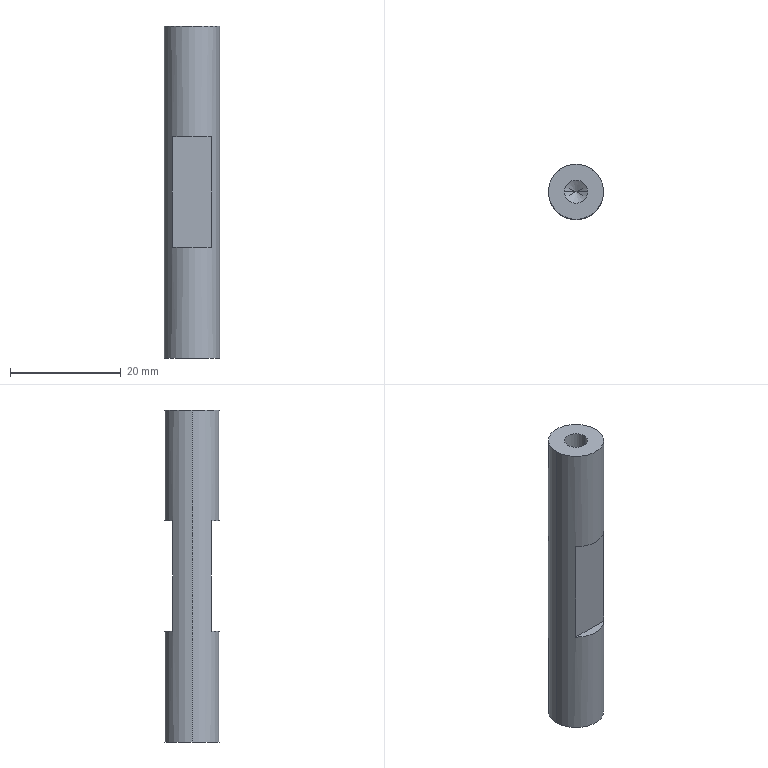Part | SolidWorks | features 3DProfileFeature 1, Extrusion 1, HoleWzd 1, ICE 1, MirrorPattern 1 | 1 solid | 18 faces | box 10 x 10 x 60 mm | volume 3990 mm3 | plane 8 | cylinder 6 | cone 4 | commonest cylinder face diameters 4.2 x4 10 x2
STEP:
#1=CARTESIAN_POINT('',(-87.9,55.,15.));
#2=VERTEX_POINT('',#1);
#3=CARTESIAN_POINT('',(-92.1,55.,15.));
#4=VERTEX_POINT('',#3);
#5=CARTESIAN_POINT('',(-90.,55.,15.));
#6=DIRECTION('',(0.,0.,-1.));
#7=DIRECTION('',(-1.,0.,0.));
#8=AXIS2_PLACEMENT_3D('',#5,#6,#7);
#9=CIRCLE('',#8,2.1);
#10=EDGE_CURVE('',#2,#4,#9,.T.);
#11=ORIENTED_EDGE('',*,*,#10,.F.);
#12=CARTESIAN_POINT('',(-87.9,55.,0.));
#13=VERTEX_POINT('',#12);
#14=CARTESIAN_POINT('',(-87.9,55.,0.));
#15=DIRECTION('',(0.,0.,-1.));
#16=VECTOR('',#15,1000.);
#17=LINE('',#14,#16);
#18=EDGE_CURVE('',#2,#13,#17,.T.);
#19=ORIENTED_EDGE('',*,*,#18,.T.);
#20=CARTESIAN_POINT('',(-92.1,55.,0.));
#21=VERTEX_POINT('',#20);
#22=CARTESIAN_POINT('',(-90.,55.,0.));
#23=DIRECTION('',(0.,0.,-1.));
#24=DIRECTION('',(-1.,0.,0.));
#25=AXIS2_PLACEMENT_3D('',#22,#23,#24);
#26=CIRCLE('',#25,2.1);
#27=EDGE_CURVE('',#13,#21,#26,.T.);
#28=ORIENTED_EDGE('',*,*,#27,.T.);
#29=CARTESIAN_POINT('',(-92.1,55.,0.));
#30=DIRECTION('',(0.,0.,-1.));
#31=VECTOR('',#30,1000.);
#32=LINE('',#29,#31);
#33=EDGE_CURVE('',#4,#21,#32,.T.);
#34=ORIENTED_EDGE('',*,*,#33,.F.);
#35=EDGE_LOOP('',(#11,#19,#28,#34));
#36=FACE_OUTER_BOUND('',#35,.T.);
#37=CARTESIAN_POINT('',(-90.,55.,0.));
#38=DIRECTION('',(0.,0.,-1.));
#39=DIRECTION('',(-1.,0.,0.));
#40=AXIS2_PLACEMENT_3D('',#37,#38,#39);
#41=CYLINDRICAL_SURFACE('',#40,2.1);
#42=ADVANCED_FACE('',(#36),#41,.F.);
#43=CARTESIAN_POINT('',(-90.,55.,16.262));
#44=VERTEX_POINT('',#43);
#45=CARTESIAN_POINT('',(-92.1,55.,15.));
#46=DIRECTION('',(-0.8572,0.,-0.515));
#47=VECTOR('',#46,1000.);
#48=LINE('',#45,#47);
#49=EDGE_CURVE('',#44,#4,#48,.T.);
#50=ORIENTED_EDGE('',*,*,#49,.F.);
#51=CARTESIAN_POINT('',(-87.9,55.,15.));
#52=DIRECTION('',(0.8572,0.,-0.515));
#53=VECTOR('',#52,1000.);
#54=LINE('',#51,#53);
#55=EDGE_CURVE('',#44,#2,#54,.T.);
#56=ORIENTED_EDGE('',*,*,#55,.T.);
#57=ORIENTED_EDGE('',*,*,#10,.T.);
#58=EDGE_LOOP('',(#50,#56,#57));
#59=FACE_OUTER_BOUND('',#58,.T.);
#60=CARTESIAN_POINT('',(-90.,55.,15.));
#61=DIRECTION('',(0.,0.,-1.));
#62=DIRECTION('',(-1.,0.,0.));
#63=AXIS2_PLACEMENT_3D('',#60,#61,#62);
#64=CONICAL_SURFACE('',#63,2.1,1.03);
#65=ADVANCED_FACE('',(#59),#64,.F.);
#66=CARTESIAN_POINT('',(-92.1,55.,45.));
#67=VERTEX_POINT('',#66);
#68=CARTESIAN_POINT('',(-87.9,55.,45.));
#69=VERTEX_POINT('',#68);
#70=CARTESIAN_POINT('',(-90.,55.,45.));
#71=DIRECTION('',(0.,0.,1.));
#72=DIRECTION('',(1.,0.,0.));
#73=AXIS2_PLACEMENT_3D('',#70,#71,#72);
#74=CIRCLE('',#73,2.1);
#75=EDGE_CURVE('',#67,#69,#74,.T.);
#76=ORIENTED_EDGE('',*,*,#75,.F.);
#77=CARTESIAN_POINT('',(-92.1,55.,60.));
#78=VERTEX_POINT('',#77);
#79=CARTESIAN_POINT('',(-92.1,55.,60.));
#80=DIRECTION('',(0.,0.,1.));
#81=VECTOR('',#80,1000.);
#82=LINE('',#79,#81);
#83=EDGE_CURVE('',#67,#78,#82,.T.);
#84=ORIENTED_EDGE('',*,*,#83,.T.);
#85=CARTESIAN_POINT('',(-87.9,55.,60.));
#86=VERTEX_POINT('',#85);
#87=CARTESIAN_POINT('',(-90.,55.,60.));
#88=DIRECTION('',(0.,0.,1.));
#89=DIRECTION('',(1.,0.,0.));
#90=AXIS2_PLACEMENT_3D('',#87,#88,#89);
#91=CIRCLE('',#90,2.1);
#92=EDGE_CURVE('',#78,#86,#91,.T.);
#93=ORIENTED_EDGE('',*,*,#92,.T.);
#94=CARTESIAN_POINT('',(-87.9,55.,60.));
#95=DIRECTION('',(0.,0.,1.));
#96=VECTOR('',#95,1000.);
#97=LINE('',#94,#96);
#98=EDGE_CURVE('',#69,#86,#97,.T.);
#99=ORIENTED_EDGE('',*,*,#98,.F.);
#100=EDGE_LOOP('',(#76,#84,#93,#99));
#101=FACE_OUTER_BOUND('',#100,.T.);
#102=CARTESIAN_POINT('',(-90.,55.,60.));
#103=DIRECTION('',(0.,0.,1.));
#104=DIRECTION('',(1.,0.,0.));
#105=AXIS2_PLACEMENT_3D('',#102,#103,#104);
#106=CYLINDRICAL_SURFACE('',#105,2.1);
#107=ADVANCED_FACE('',(#101),#106,.F.);
#108=CARTESIAN_POINT('',(-90.,55.,43.738));
#109=VERTEX_POINT('',#108);
#110=CARTESIAN_POINT('',(-87.9,55.,45.));
#111=DIRECTION('',(0.8572,0.,0.515));
#112=VECTOR('',#111,1000.);
#113=LINE('',#110,#112);
#114=EDGE_CURVE('',#109,#69,#113,.T.);
#115=ORIENTED_EDGE('',*,*,#114,.F.);
#116=CARTESIAN_POINT('',(-92.1,55.,45.));
#117=DIRECTION('',(-0.8572,0.,0.515));
#118=VECTOR('',#117,1000.);
#119=LINE('',#116,#118);
#120=EDGE_CURVE('',#109,#67,#119,.T.);
#121=ORIENTED_EDGE('',*,*,#120,.T.);
#122=ORIENTED_EDGE('',*,*,#75,.T.);
#123=EDGE_LOOP('',(#115,#121,#122));
#124=FACE_OUTER_BOUND('',#123,.T.);
#125=CARTESIAN_POINT('',(-90.,55.,45.));
#126=DIRECTION('',(0.,0.,1.));
#127=DIRECTION('',(1.,0.,0.));
#128=AXIS2_PLACEMENT_3D('',#125,#126,#127);
#129=CONICAL_SURFACE('',#128,2.1,1.03);
#130=ADVANCED_FACE('',(#124),#129,.F.);
#131=CARTESIAN_POINT('',(-86.429,58.5,20.));
#132=VERTEX_POINT('',#131);
#133=CARTESIAN_POINT('',(-86.429,58.5,40.));
#134=VERTEX_POINT('',#133);
#135=CARTESIAN_POINT('',(-86.429,58.5,60.));
#136=DIRECTION('',(0.,0.,1.));
#137=VECTOR('',#136,1000.);
#138=LINE('',#135,#137);
#139=EDGE_CURVE('',#132,#134,#138,.T.);
#140=ORIENTED_EDGE('',*,*,#139,.T.);
#141=CARTESIAN_POINT('',(-93.571,58.5,40.));
#142=VERTEX_POINT('',#141);
#143=CARTESIAN_POINT('',(-90.,55.,40.));
#144=DIRECTION('',(0.,0.,1.));
#145=DIRECTION('',(1.,0.,0.));
#146=AXIS2_PLACEMENT_3D('',#143,#144,#145);
#147=CIRCLE('',#146,5.);
#148=EDGE_CURVE('',#134,#142,#147,.T.);
#149=ORIENTED_EDGE('',*,*,#148,.T.);
#150=CARTESIAN_POINT('',(-93.571,58.5,20.));
#151=VERTEX_POINT('',#150);
#152=CARTESIAN_POINT('',(-93.571,58.5,60.));
#153=DIRECTION('',(0.,0.,-1.));
#154=VECTOR('',#153,1000.);
#155=LINE('',#152,#154);
#156=EDGE_CURVE('',#142,#151,#155,.T.);
#157=ORIENTED_EDGE('',*,*,#156,.T.);
#158=CARTESIAN_POINT('',(-90.,55.,20.));
#159=DIRECTION('',(0.,0.,-1.));
#160=DIRECTION('',(-1.,0.,0.));
#161=AXIS2_PLACEMENT_3D('',#158,#159,#160);
#162=CIRCLE('',#161,5.);
#163=EDGE_CURVE('',#151,#132,#162,.T.);
#164=ORIENTED_EDGE('',*,*,#163,.T.);
#165=EDGE_LOOP('',(#140,#149,#157,#164));
#166=FACE_BOUND('',#165,.T.);
#167=CARTESIAN_POINT('',(-85.,55.,60.));
#168=VERTEX_POINT('',#167);
#169=CARTESIAN_POINT('',(-95.,55.,60.));
#170=VERTEX_POINT('',#169);
#171=CARTESIAN_POINT('',(-90.,55.,60.));
#172=DIRECTION('',(0.,0.,1.));
#173=DIRECTION('',(1.,0.,0.));
#174=AXIS2_PLACEMENT_3D('',#171,#172,#173);
#175=CIRCLE('',#174,5.);
#176=EDGE_CURVE('',#168,#170,#175,.T.);
#177=ORIENTED_EDGE('',*,*,#176,.F.);
#178=CARTESIAN_POINT('',(-85.,55.,0.));
#179=VERTEX_POINT('',#178);
#180=CARTESIAN_POINT('',(-85.,55.,60.));
#181=DIRECTION('',(0.,0.,-1.));
#182=VECTOR('',#181,1000.);
#183=LINE('',#180,#182);
#184=EDGE_CURVE('',#168,#179,#183,.T.);
#185=ORIENTED_EDGE('',*,*,#184,.T.);
#186=CARTESIAN_POINT('',(-95.,55.,0.));
#187=VERTEX_POINT('',#186);
#188=CARTESIAN_POINT('',(-90.,55.,0.));
#189=DIRECTION('',(0.,0.,1.));
#190=DIRECTION('',(1.,0.,0.));
#191=AXIS2_PLACEMENT_3D('',#188,#189,#190);
#192=CIRCLE('',#191,5.);
#193=EDGE_CURVE('',#179,#187,#192,.T.);
#194=ORIENTED_EDGE('',*,*,#193,.T.);
#195=CARTESIAN_POINT('',(-95.,55.,60.));
#196=DIRECTION('',(0.,0.,-1.));
#197=VECTOR('',#196,1000.);
#198=LINE('',#195,#197);
#199=EDGE_CURVE('',#170,#187,#198,.T.);
#200=ORIENTED_EDGE('',*,*,#199,.F.);
#201=EDGE_LOOP('',(#177,#185,#194,#200));
#202=FACE_OUTER_BOUND('',#201,.T.);
#203=CARTESIAN_POINT('',(-90.,55.,60.));
#204=DIRECTION('',(0.,0.,-1.));
#205=DIRECTION('',(-1.,0.,0.));
#206=AXIS2_PLACEMENT_3D('',#203,#204,#205);
#207=CYLINDRICAL_SURFACE('',#206,5.);
#208=ADVANCED_FACE('',(#166,#202),#207,.T.);
#209=ORIENTED_EDGE('',*,*,#184,.F.);
#210=CARTESIAN_POINT('',(-90.,55.,60.));
#211=DIRECTION('',(0.,0.,1.));
#212=DIRECTION('',(1.,0.,0.));
#213=AXIS2_PLACEMENT_3D('',#210,#211,#212);
#214=CIRCLE('',#213,5.);
#215=EDGE_CURVE('',#170,#168,#214,.T.);
#216=ORIENTED_EDGE('',*,*,#215,.F.);
#217=ORIENTED_EDGE('',*,*,#199,.T.);
#218=CARTESIAN_POINT('',(-90.,55.,0.));
#219=DIRECTION('',(0.,0.,1.));
#220=DIRECTION('',(1.,0.,0.));
#221=AXIS2_PLACEMENT_3D('',#218,#219,#220);
#222=CIRCLE('',#221,5.);
#223=EDGE_CURVE('',#187,#179,#222,.T.);
#224=ORIENTED_EDGE('',*,*,#223,.T.);
#225=EDGE_LOOP('',(#209,#216,#217,#224));
#226=FACE_OUTER_BOUND('',#225,.T.);
#227=CARTESIAN_POINT('',(-93.571,51.5,20.));
#228=VERTEX_POINT('',#227);
#229=CARTESIAN_POINT('',(-86.429,51.5,20.));
#230=VERTEX_POINT('',#229);
#231=CARTESIAN_POINT('',(-90.,55.,20.));
#232=DIRECTION('',(0.,0.,1.));
#233=DIRECTION('',(1.,0.,0.));
#234=AXIS2_PLACEMENT_3D('',#231,#232,#233);
#235=CIRCLE('',#234,5.);
#236=EDGE_CURVE('',#228,#230,#235,.T.);
#237=ORIENTED_EDGE('',*,*,#236,.F.);
#238=CARTESIAN_POINT('',(-93.571,51.5,40.));
#239=VERTEX_POINT('',#238);
#240=CARTESIAN_POINT('',(-93.571,51.5,60.));
#241=DIRECTION('',(0.,0.,1.));
#242=VECTOR('',#241,1000.);
#243=LINE('',#240,#242);
#244=EDGE_CURVE('',#228,#239,#243,.T.);
#245=ORIENTED_EDGE('',*,*,#244,.T.);
#246=CARTESIAN_POINT('',(-86.429,51.5,40.));
#247=VERTEX_POINT('',#246);
#248=CARTESIAN_POINT('',(-90.,55.,40.));
#249=DIRECTION('',(0.,0.,-1.));
#250=DIRECTION('',(-1.,0.,0.));
#251=AXIS2_PLACEMENT_3D('',#248,#249,#250);
#252=CIRCLE('',#251,5.);
#253=EDGE_CURVE('',#247,#239,#252,.T.);
#254=ORIENTED_EDGE('',*,*,#253,.F.);
#255=CARTESIAN_POINT('',(-86.429,51.5,60.));
#256=DIRECTION('',(0.,0.,-1.));
#257=VECTOR('',#256,1000.);
#258=LINE('',#255,#257);
#259=EDGE_CURVE('',#247,#230,#258,.T.);
#260=ORIENTED_EDGE('',*,*,#259,.T.);
#261=EDGE_LOOP('',(#237,#245,#254,#260));
#262=FACE_BOUND('',#261,.T.);
#263=CARTESIAN_POINT('',(-90.,55.,60.));
#264=DIRECTION('',(0.,0.,-1.));
#265=DIRECTION('',(-1.,0.,0.));
#266=AXIS2_PLACEMENT_3D('',#263,#264,#265);
#267=CYLINDRICAL_SURFACE('',#266,5.);
#268=ADVANCED_FACE('',(#226,#262),#267,.T.);
#269=CARTESIAN_POINT('',(-90.,55.,60.));
#270=DIRECTION('',(0.,0.,1.));
#271=DIRECTION('',(1.,0.,0.));
#272=AXIS2_PLACEMENT_3D('',#269,#270,#271);
#273=CIRCLE('',#272,2.1);
#274=EDGE_CURVE('',#86,#78,#273,.T.);
#275=ORIENTED_EDGE('',*,*,#274,.F.);
#276=ORIENTED_EDGE('',*,*,#92,.F.);
#277=EDGE_LOOP('',(#275,#276));
#278=FACE_BOUND('',#277,.T.);
#279=ORIENTED_EDGE('',*,*,#215,.T.);
#280=ORIENTED_EDGE('',*,*,#176,.T.);
#281=EDGE_LOOP('',(#279,#280));
#282=FACE_OUTER_BOUND('',#281,.T.);
#283=CARTESIAN_POINT('',(-90.,55.,60.));
#284=DIRECTION('',(0.,0.,1.));
#285=DIRECTION('',(1.,0.,0.));
#286=AXIS2_PLACEMENT_3D('',#283,#284,#285);
#287=PLANE('',#286);
#288=ADVANCED_FACE('',(#278,#282),#287,.T.);
#289=CARTESIAN_POINT('',(-90.,55.,0.));
#290=DIRECTION('',(0.,0.,-1.));
#291=DIRECTION('',(-1.,0.,0.));
#292=AXIS2_PLACEMENT_3D('',#289,#290,#291);
#293=CIRCLE('',#292,2.1);
#294=EDGE_CURVE('',#21,#13,#293,.T.);
#295=ORIENTED_EDGE('',*,*,#294,.F.);
#296=ORIENTED_EDGE('',*,*,#27,.F.);
#297=EDGE_LOOP('',(#295,#296));
#298=FACE_BOUND('',#297,.T.);
#299=ORIENTED_EDGE('',*,*,#223,.F.);
#300=ORIENTED_EDGE('',*,*,#193,.F.);
#301=EDGE_LOOP('',(#299,#300));
#302=FACE_OUTER_BOUND('',#301,.T.);
#303=CARTESIAN_POINT('',(-90.,55.,0.));
#304=DIRECTION('',(0.,0.,1.));
#305=DIRECTION('',(1.,0.,0.));
#306=AXIS2_PLACEMENT_3D('',#303,#304,#305);
#307=PLANE('',#306);
#308=ADVANCED_FACE('',(#298,#302),#307,.F.);
#309=CARTESIAN_POINT('',(-100.,58.5,40.));
#310=DIRECTION('',(1.,0.,0.));
#311=VECTOR('',#310,1000.);
#312=LINE('',#309,#311);
#313=EDGE_CURVE('',#142,#134,#312,.T.);
#314=ORIENTED_EDGE('',*,*,#313,.F.);
#315=ORIENTED_EDGE('',*,*,#148,.F.);
#316=EDGE_LOOP('',(#314,#315));
#317=FACE_OUTER_BOUND('',#316,.T.);
#318=CARTESIAN_POINT('',(-100.,58.5,40.));
#319=DIRECTION('',(0.,0.,1.));
#320=DIRECTION('',(1.,0.,0.));
#321=AXIS2_PLACEMENT_3D('',#318,#319,#320);
#322=PLANE('',#321);
#323=ADVANCED_FACE('',(#317),#322,.F.);
#324=CARTESIAN_POINT('',(-100.,58.5,20.));
#325=DIRECTION('',(-1.,0.,0.));
#326=VECTOR('',#325,1000.);
#327=LINE('',#324,#326);
#328=EDGE_CURVE('',#132,#151,#327,.T.);
#329=ORIENTED_EDGE('',*,*,#328,.F.);
#330=ORIENTED_EDGE('',*,*,#163,.F.);
#331=EDGE_LOOP('',(#329,#330));
#332=FACE_OUTER_BOUND('',#331,.T.);
#333=CARTESIAN_POINT('',(-100.,58.5,20.));
#334=DIRECTION('',(0.,0.,-1.));
#335=DIRECTION('',(-1.,0.,0.));
#336=AXIS2_PLACEMENT_3D('',#333,#334,#335);
#337=PLANE('',#336);
#338=ADVANCED_FACE('',(#332),#337,.F.);
#339=ORIENTED_EDGE('',*,*,#313,.T.);
#340=ORIENTED_EDGE('',*,*,#139,.F.);
#341=ORIENTED_EDGE('',*,*,#328,.T.);
#342=ORIENTED_EDGE('',*,*,#156,.F.);
#343=EDGE_LOOP('',(#339,#340,#341,#342));
#344=FACE_OUTER_BOUND('',#343,.T.);
#345=CARTESIAN_POINT('',(0.,58.5,0.));
#346=DIRECTION('',(0.,-1.,0.));
#347=DIRECTION('',(0.,0.,-1.));
#348=AXIS2_PLACEMENT_3D('',#345,#346,#347);
#349=PLANE('',#348);
#350=ADVANCED_FACE('',(#344),#349,.F.);
#351=CARTESIAN_POINT('',(-100.,51.5,20.));
#352=DIRECTION('',(-1.,0.,0.));
#353=VECTOR('',#352,1000.);
#354=LINE('',#351,#353);
#355=EDGE_CURVE('',#230,#228,#354,.T.);
#356=ORIENTED_EDGE('',*,*,#355,.T.);
#357=ORIENTED_EDGE('',*,*,#236,.T.);
#358=EDGE_LOOP('',(#356,#357));
#359=FACE_OUTER_BOUND('',#358,.T.);
#360=CARTESIAN_POINT('',(-100.,51.5,20.));
#361=DIRECTION('',(0.,0.,1.));
#362=DIRECTION('',(1.,0.,0.));
#363=AXIS2_PLACEMENT_3D('',#360,#361,#362);
#364=PLANE('',#363);
#365=ADVANCED_FACE('',(#359),#364,.T.);
#366=CARTESIAN_POINT('',(-100.,51.5,40.));
#367=DIRECTION('',(1.,0.,0.));
#368=VECTOR('',#367,1000.);
#369=LINE('',#366,#368);
#370=EDGE_CURVE('',#239,#247,#369,.T.);
#371=ORIENTED_EDGE('',*,*,#370,.T.);
#372=ORIENTED_EDGE('',*,*,#253,.T.);
#373=EDGE_LOOP('',(#371,#372));
#374=FACE_OUTER_BOUND('',#373,.T.);
#375=CARTESIAN_POINT('',(-100.,51.5,40.));
#376=DIRECTION('',(0.,0.,-1.));
#377=DIRECTION('',(-1.,0.,0.));
#378=AXIS2_PLACEMENT_3D('',#375,#376,#377);
#379=PLANE('',#378);
#380=ADVANCED_FACE('',(#374),#379,.T.);
#381=ORIENTED_EDGE('',*,*,#370,.F.);
#382=ORIENTED_EDGE('',*,*,#244,.F.);
#383=ORIENTED_EDGE('',*,*,#355,.F.);
#384=ORIENTED_EDGE('',*,*,#259,.F.);
#385=EDGE_LOOP('',(#381,#382,#383,#384));
#386=FACE_OUTER_BOUND('',#385,.T.);
#387=CARTESIAN_POINT('',(0.,51.5,0.));
#388=DIRECTION('',(0.,1.,0.));
#389=DIRECTION('',(0.,0.,-1.));
#390=AXIS2_PLACEMENT_3D('',#387,#388,#389);
#391=PLANE('',#390);
#392=ADVANCED_FACE('',(#386),#391,.F.);
#393=ORIENTED_EDGE('',*,*,#120,.F.);
#394=ORIENTED_EDGE('',*,*,#114,.T.);
#395=CARTESIAN_POINT('',(-90.,55.,45.));
#396=DIRECTION('',(0.,0.,1.));
#397=DIRECTION('',(1.,0.,0.));
#398=AXIS2_PLACEMENT_3D('',#395,#396,#397);
#399=CIRCLE('',#398,2.1);
#400=EDGE_CURVE('',#69,#67,#399,.T.);
#401=ORIENTED_EDGE('',*,*,#400,.T.);
#402=EDGE_LOOP('',(#393,#394,#401));
#403=FACE_OUTER_BOUND('',#402,.T.);
#404=CARTESIAN_POINT('',(-90.,55.,45.));
#405=DIRECTION('',(0.,0.,1.));
#406=DIRECTION('',(1.,0.,0.));
#407=AXIS2_PLACEMENT_3D('',#404,#405,#406);
#408=CONICAL_SURFACE('',#407,2.1,1.03);
#409=ADVANCED_FACE('',(#403),#408,.F.);
#410=ORIENTED_EDGE('',*,*,#83,.F.);
#411=ORIENTED_EDGE('',*,*,#400,.F.);
#412=ORIENTED_EDGE('',*,*,#98,.T.);
#413=ORIENTED_EDGE('',*,*,#274,.T.);
#414=EDGE_LOOP('',(#410,#411,#412,#413));
#415=FACE_OUTER_BOUND('',#414,.T.);
#416=CARTESIAN_POINT('',(-90.,55.,60.));
#417=DIRECTION('',(0.,0.,1.));
#418=DIRECTION('',(1.,0.,0.));
#419=AXIS2_PLACEMENT_3D('',#416,#417,#418);
#420=CYLINDRICAL_SURFACE('',#419,2.1);
#421=ADVANCED_FACE('',(#415),#420,.F.);
#422=ORIENTED_EDGE('',*,*,#55,.F.);
#423=ORIENTED_EDGE('',*,*,#49,.T.);
#424=CARTESIAN_POINT('',(-90.,55.,15.));
#425=DIRECTION('',(0.,0.,-1.));
#426=DIRECTION('',(-1.,0.,0.));
#427=AXIS2_PLACEMENT_3D('',#424,#425,#426);
#428=CIRCLE('',#427,2.1);
#429=EDGE_CURVE('',#4,#2,#428,.T.);
#430=ORIENTED_EDGE('',*,*,#429,.T.);
#431=EDGE_LOOP('',(#422,#423,#430));
#432=FACE_OUTER_BOUND('',#431,.T.);
#433=CARTESIAN_POINT('',(-90.,55.,15.));
#434=DIRECTION('',(0.,0.,-1.));
#435=DIRECTION('',(-1.,0.,0.));
#436=AXIS2_PLACEMENT_3D('',#433,#434,#435);
#437=CONICAL_SURFACE('',#436,2.1,1.03);
#438=ADVANCED_FACE('',(#432),#437,.F.);
#439=ORIENTED_EDGE('',*,*,#18,.F.);
#440=ORIENTED_EDGE('',*,*,#429,.F.);
#441=ORIENTED_EDGE('',*,*,#33,.T.);
#442=ORIENTED_EDGE('',*,*,#294,.T.);
#443=EDGE_LOOP('',(#439,#440,#441,#442));
#444=FACE_OUTER_BOUND('',#443,.T.);
#445=CARTESIAN_POINT('',(-90.,55.,0.));
#446=DIRECTION('',(0.,0.,-1.));
#447=DIRECTION('',(-1.,0.,0.));
#448=AXIS2_PLACEMENT_3D('',#445,#446,#447);
#449=CYLINDRICAL_SURFACE('',#448,2.1);
#450=ADVANCED_FACE('',(#444),#449,.F.);
#451=CLOSED_SHELL('',(#42,#65,#107,#130,#208,#268,#288,#308,#323,#338,#350,#365,#380,#392,#409,#421,#438,#450));
#452=MANIFOLD_SOLID_BREP('',#451);
#453=CARTESIAN_POINT('',(0.,0.,0.));
#454=DIRECTION('',(0.,0.,1.));
#455=DIRECTION('',(1.,0.,0.));
#456=AXIS2_PLACEMENT_3D('',#453,#454,#455);
#457=(LENGTH_UNIT()NAMED_UNIT(*)SI_UNIT(.MILLI.,.METRE.));
#458=UNCERTAINTY_MEASURE_WITH_UNIT(LENGTH_MEASURE(0.00001),#457,'','');
#459=(NAMED_UNIT(*)PLANE_ANGLE_UNIT()SI_UNIT($,.RADIAN.));
#460=(NAMED_UNIT(*)SI_UNIT($,.STERADIAN.)SOLID_ANGLE_UNIT());
#461=(GEOMETRIC_REPRESENTATION_CONTEXT(3)GLOBAL_UNCERTAINTY_ASSIGNED_CONTEXT((#458))GLOBAL_UNIT_ASSIGNED_CONTEXT((#457,#459,#460))REPRESENTATION_CONTEXT('',''));
#462=ADVANCED_BREP_SHAPE_REPRESENTATION('',(#452,#456),#461);